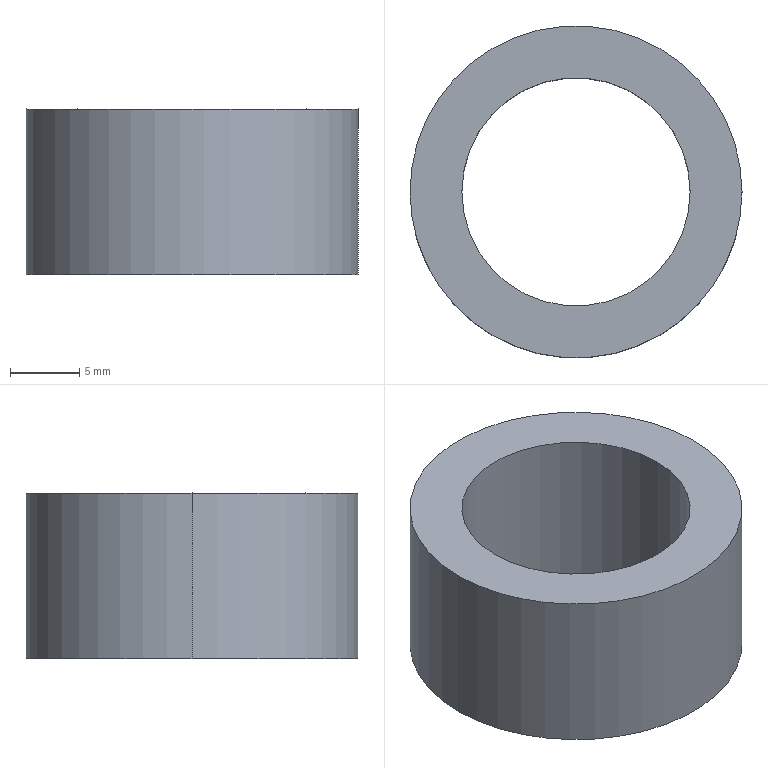Part | SolidWorks | features Extrusion 1 | 1 solid | 6 faces | box 24 x 24 x 12 mm | volume 2863 mm3 | cylinder 4 | plane 2 | commonest cylinder face diameters 16.5 x2 24 x2
STEP:
#1=CARTESIAN_POINT('',(-8.25,0.,12.));
#2=VERTEX_POINT('',#1);
#3=CARTESIAN_POINT('',(8.25,0.,12.));
#4=VERTEX_POINT('',#3);
#5=CARTESIAN_POINT('',(0.,0.,12.));
#6=DIRECTION('',(0.,0.,1.));
#7=DIRECTION('',(1.,0.,0.));
#8=AXIS2_PLACEMENT_3D('',#5,#6,#7);
#9=CIRCLE('',#8,8.25);
#10=EDGE_CURVE('',#2,#4,#9,.T.);
#11=ORIENTED_EDGE('',*,*,#10,.T.);
#12=CARTESIAN_POINT('',(8.25,0.,0.));
#13=VERTEX_POINT('',#12);
#14=CARTESIAN_POINT('',(8.25,0.,12.));
#15=DIRECTION('',(0.,0.,-1.));
#16=VECTOR('',#15,1000.);
#17=LINE('',#14,#16);
#18=EDGE_CURVE('',#4,#13,#17,.T.);
#19=ORIENTED_EDGE('',*,*,#18,.T.);
#20=CARTESIAN_POINT('',(-8.25,0.,0.));
#21=VERTEX_POINT('',#20);
#22=CARTESIAN_POINT('',(0.,0.,0.));
#23=DIRECTION('',(0.,0.,1.));
#24=DIRECTION('',(1.,0.,0.));
#25=AXIS2_PLACEMENT_3D('',#22,#23,#24);
#26=CIRCLE('',#25,8.25);
#27=EDGE_CURVE('',#21,#13,#26,.T.);
#28=ORIENTED_EDGE('',*,*,#27,.F.);
#29=CARTESIAN_POINT('',(-8.25,0.,12.));
#30=DIRECTION('',(0.,0.,-1.));
#31=VECTOR('',#30,1000.);
#32=LINE('',#29,#31);
#33=EDGE_CURVE('',#2,#21,#32,.T.);
#34=ORIENTED_EDGE('',*,*,#33,.F.);
#35=EDGE_LOOP('',(#11,#19,#28,#34));
#36=FACE_OUTER_BOUND('',#35,.T.);
#37=CARTESIAN_POINT('',(0.,0.,12.));
#38=DIRECTION('',(0.,0.,-1.));
#39=DIRECTION('',(-1.,0.,0.));
#40=AXIS2_PLACEMENT_3D('',#37,#38,#39);
#41=CYLINDRICAL_SURFACE('',#40,8.25);
#42=ADVANCED_FACE('',(#36),#41,.F.);
#43=CARTESIAN_POINT('',(12.,0.,12.));
#44=VERTEX_POINT('',#43);
#45=CARTESIAN_POINT('',(-12.,0.,12.));
#46=VERTEX_POINT('',#45);
#47=CARTESIAN_POINT('',(0.,0.,12.));
#48=DIRECTION('',(0.,0.,1.));
#49=DIRECTION('',(1.,0.,0.));
#50=AXIS2_PLACEMENT_3D('',#47,#48,#49);
#51=CIRCLE('',#50,12.);
#52=EDGE_CURVE('',#44,#46,#51,.T.);
#53=ORIENTED_EDGE('',*,*,#52,.F.);
#54=CARTESIAN_POINT('',(12.,0.,0.));
#55=VERTEX_POINT('',#54);
#56=CARTESIAN_POINT('',(12.,0.,12.));
#57=DIRECTION('',(0.,0.,-1.));
#58=VECTOR('',#57,1000.);
#59=LINE('',#56,#58);
#60=EDGE_CURVE('',#44,#55,#59,.T.);
#61=ORIENTED_EDGE('',*,*,#60,.T.);
#62=CARTESIAN_POINT('',(-12.,0.,0.));
#63=VERTEX_POINT('',#62);
#64=CARTESIAN_POINT('',(0.,0.,0.));
#65=DIRECTION('',(0.,0.,1.));
#66=DIRECTION('',(1.,0.,0.));
#67=AXIS2_PLACEMENT_3D('',#64,#65,#66);
#68=CIRCLE('',#67,12.);
#69=EDGE_CURVE('',#55,#63,#68,.T.);
#70=ORIENTED_EDGE('',*,*,#69,.T.);
#71=CARTESIAN_POINT('',(-12.,0.,12.));
#72=DIRECTION('',(0.,0.,-1.));
#73=VECTOR('',#72,1000.);
#74=LINE('',#71,#73);
#75=EDGE_CURVE('',#46,#63,#74,.T.);
#76=ORIENTED_EDGE('',*,*,#75,.F.);
#77=EDGE_LOOP('',(#53,#61,#70,#76));
#78=FACE_OUTER_BOUND('',#77,.T.);
#79=CARTESIAN_POINT('',(0.,0.,12.));
#80=DIRECTION('',(0.,0.,-1.));
#81=DIRECTION('',(-1.,0.,0.));
#82=AXIS2_PLACEMENT_3D('',#79,#80,#81);
#83=CYLINDRICAL_SURFACE('',#82,12.);
#84=ADVANCED_FACE('',(#78),#83,.T.);
#85=CARTESIAN_POINT('',(0.,0.,12.));
#86=DIRECTION('',(0.,0.,1.));
#87=DIRECTION('',(1.,0.,0.));
#88=AXIS2_PLACEMENT_3D('',#85,#86,#87);
#89=CIRCLE('',#88,12.);
#90=EDGE_CURVE('',#46,#44,#89,.T.);
#91=ORIENTED_EDGE('',*,*,#90,.T.);
#92=ORIENTED_EDGE('',*,*,#52,.T.);
#93=EDGE_LOOP('',(#91,#92));
#94=FACE_OUTER_BOUND('',#93,.T.);
#95=ORIENTED_EDGE('',*,*,#10,.F.);
#96=CARTESIAN_POINT('',(0.,0.,12.));
#97=DIRECTION('',(0.,0.,1.));
#98=DIRECTION('',(1.,0.,0.));
#99=AXIS2_PLACEMENT_3D('',#96,#97,#98);
#100=CIRCLE('',#99,8.25);
#101=EDGE_CURVE('',#4,#2,#100,.T.);
#102=ORIENTED_EDGE('',*,*,#101,.F.);
#103=EDGE_LOOP('',(#95,#102));
#104=FACE_BOUND('',#103,.T.);
#105=CARTESIAN_POINT('',(0.,0.,12.));
#106=DIRECTION('',(0.,0.,1.));
#107=DIRECTION('',(1.,0.,0.));
#108=AXIS2_PLACEMENT_3D('',#105,#106,#107);
#109=PLANE('',#108);
#110=ADVANCED_FACE('',(#94,#104),#109,.T.);
#111=CARTESIAN_POINT('',(0.,0.,0.));
#112=DIRECTION('',(0.,0.,1.));
#113=DIRECTION('',(1.,0.,0.));
#114=AXIS2_PLACEMENT_3D('',#111,#112,#113);
#115=CIRCLE('',#114,12.);
#116=EDGE_CURVE('',#63,#55,#115,.T.);
#117=ORIENTED_EDGE('',*,*,#116,.F.);
#118=ORIENTED_EDGE('',*,*,#69,.F.);
#119=EDGE_LOOP('',(#117,#118));
#120=FACE_OUTER_BOUND('',#119,.T.);
#121=ORIENTED_EDGE('',*,*,#27,.T.);
#122=CARTESIAN_POINT('',(0.,0.,0.));
#123=DIRECTION('',(0.,0.,1.));
#124=DIRECTION('',(1.,0.,0.));
#125=AXIS2_PLACEMENT_3D('',#122,#123,#124);
#126=CIRCLE('',#125,8.25);
#127=EDGE_CURVE('',#13,#21,#126,.T.);
#128=ORIENTED_EDGE('',*,*,#127,.T.);
#129=EDGE_LOOP('',(#121,#128));
#130=FACE_BOUND('',#129,.T.);
#131=CARTESIAN_POINT('',(0.,0.,0.));
#132=DIRECTION('',(0.,0.,1.));
#133=DIRECTION('',(1.,0.,0.));
#134=AXIS2_PLACEMENT_3D('',#131,#132,#133);
#135=PLANE('',#134);
#136=ADVANCED_FACE('',(#120,#130),#135,.F.);
#137=ORIENTED_EDGE('',*,*,#60,.F.);
#138=ORIENTED_EDGE('',*,*,#90,.F.);
#139=ORIENTED_EDGE('',*,*,#75,.T.);
#140=ORIENTED_EDGE('',*,*,#116,.T.);
#141=EDGE_LOOP('',(#137,#138,#139,#140));
#142=FACE_OUTER_BOUND('',#141,.T.);
#143=CARTESIAN_POINT('',(0.,0.,12.));
#144=DIRECTION('',(0.,0.,-1.));
#145=DIRECTION('',(-1.,0.,0.));
#146=AXIS2_PLACEMENT_3D('',#143,#144,#145);
#147=CYLINDRICAL_SURFACE('',#146,12.);
#148=ADVANCED_FACE('',(#142),#147,.T.);
#149=ORIENTED_EDGE('',*,*,#18,.F.);
#150=ORIENTED_EDGE('',*,*,#101,.T.);
#151=ORIENTED_EDGE('',*,*,#33,.T.);
#152=ORIENTED_EDGE('',*,*,#127,.F.);
#153=EDGE_LOOP('',(#149,#150,#151,#152));
#154=FACE_OUTER_BOUND('',#153,.T.);
#155=CARTESIAN_POINT('',(0.,0.,12.));
#156=DIRECTION('',(0.,0.,-1.));
#157=DIRECTION('',(-1.,0.,0.));
#158=AXIS2_PLACEMENT_3D('',#155,#156,#157);
#159=CYLINDRICAL_SURFACE('',#158,8.25);
#160=ADVANCED_FACE('',(#154),#159,.F.);
#161=CLOSED_SHELL('',(#42,#84,#110,#136,#148,#160));
#162=MANIFOLD_SOLID_BREP('',#161);
#163=CARTESIAN_POINT('',(0.,0.,0.));
#164=DIRECTION('',(0.,0.,1.));
#165=DIRECTION('',(1.,0.,0.));
#166=AXIS2_PLACEMENT_3D('',#163,#164,#165);
#167=(LENGTH_UNIT()NAMED_UNIT(*)SI_UNIT(.MILLI.,.METRE.));
#168=UNCERTAINTY_MEASURE_WITH_UNIT(LENGTH_MEASURE(0.00001),#167,'','');
#169=(NAMED_UNIT(*)PLANE_ANGLE_UNIT()SI_UNIT($,.RADIAN.));
#170=(NAMED_UNIT(*)SI_UNIT($,.STERADIAN.)SOLID_ANGLE_UNIT());
#171=(GEOMETRIC_REPRESENTATION_CONTEXT(3)GLOBAL_UNCERTAINTY_ASSIGNED_CONTEXT((#168))GLOBAL_UNIT_ASSIGNED_CONTEXT((#167,#169,#170))REPRESENTATION_CONTEXT('',''));
#172=ADVANCED_BREP_SHAPE_REPRESENTATION('',(#162,#166),#171);